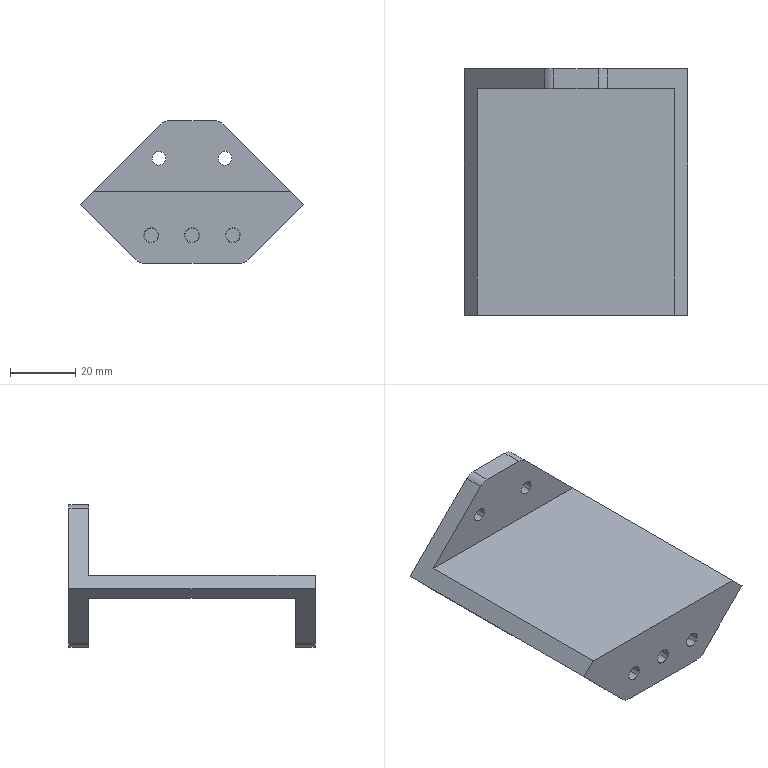NC program | NX | posted with a generic post | part box 68.307 x 75.3 x 43.668 mm
Lines 2926 to 4118 of 6865:
(ZLEVEL_PROFILE_1_COPY_1 , TOOL : D6R0.5)
N5832 T16 M6
N5834 G54
N5836 G17 G0 G90 X-11.309 Y27.842 B0. C0. S9500 M3
N5838 G43 Z30. H16
N5840 Z2.995
N5842 G94 G1 Z-0.005 F3500.
N5844 G3 X-9.487 Y31.148 R3.
N5846 G1 X-9.496 Y31.178
N5848 X-9.541 Y31.65
N5850 Y37.65
N5852 X-9.485 Y38.151
N5854 X-9.538 Y38.15 Z-0.008
N5856 X-9.549 Z-0.01
N5858 X-9.628 Y37.65
N5860 Y31.65
N5862 G3 X-9.55 Y31.15 R3.795
N5864 G1 X-9.633 Z-0.014
N5866 X-9.649 Z-0.019
N5868 X-9.738 Y31.65
N5870 Y37.65
N5872 X-9.648 Y38.15
N5874 X-9.719 Z-0.022
N5876 X-9.718 Z-0.025
N5878 X-9.8 Y37.65
N5880 Y31.65
N5882 G3 X-9.719 Y31.15 R2.274
N5884 G1 X-9.787 Z-0.031
N5886 X-9.852 Y31.65
N5888 Y37.65
N5890 X-9.785 Y38.149
N5892 X-9.833 Y38.15 Z-0.034
N5894 X-9.858 Z-0.038
N5896 X-9.915 Y37.65
N5898 Y31.65
N5900 X-9.857 Y31.15
N5902 X-9.903 Y31.151 Z-0.044
N5904 X-9.919 Z-0.049
N5906 X-9.99 Y31.65
N5908 Y37.65
N5910 X-9.921 Y38.15
N5912 X-9.984 Z-0.056
N5914 X-10.005 Z-0.063
N5916 X-10.077 Y37.65
N5918 Y31.65
N5920 X-10.003 Y31.151
N5922 X-10.104 Z-0.08
N5924 X-10.171 Y31.65
N5926 Y37.65
N5928 X-10.107 Y38.15
N5930 X-10.173 Z-0.089
N5932 X-10.215 Z-0.099
N5934 X-10.269 Y37.65
N5936 Y31.65
N5938 X-10.258 Y31.627
N5940 X-10.227 Y31.203
N5942 X-10.215 Y31.136
N5944 X-10.263 Y31.13 Z-0.11
N5946 X-10.307 Y31.125 Z-0.121
N5948 X-10.363 Y31.65
N5950 Y37.65
N5952 X-10.303 Y38.15
N5954 X-10.308 Y38.256 Z-0.125
N5956 X-10.301 Y38.36 Z-0.129
N5958 X-10.302 Y38.354
N5960 X-10.338 Y38.151
N5962 G3 X-10.399 Y37.65 R2.023
N5964 G1 Y31.65
N5966 X-10.339 Y31.098
N5968 X-10.313 Y31.017
N5970 X-10.356 Y31.015 Z-0.138
N5972 X-10.382 Y31.013 Z-0.147
N5974 X-10.416 Y31.134
N5976 X-10.471 Y31.65
N5978 Y37.65
N5980 X-10.411 Y38.15
N5982 X-10.369 Y38.37
N5984 X-10.314 Y38.541
N5986 X-10.386 Y38.411 Z-0.156
N5988 X-10.456 Y38.282 Z-0.165
N5990 X-10.517 Y38.15 Z-0.174
N5992 X-10.532 Y38.078
N5994 X-10.567 Y37.65
N5996 Y31.65
N5998 X-10.513 Y31.123
N6000 X-10.481 Y31.007
N6002 X-10.551 Y31.074 Z-0.188
N6004 X-10.611 Y31.146 Z-0.202
N6006 X-10.615 Y31.152
N6008 X-10.651 Y31.627
N6010 X-10.663 Y31.65
N6012 Y37.65
N6014 X-10.604 Y38.159
N6016 X-10.659 Y38.167 Z-0.218
N6018 X-10.694 Y38.171 Z-0.233
N6020 X-10.757 Y37.65
N6022 Y31.65
N6024 X-10.746 Y31.627
N6026 X-10.708 Y31.145
N6028 X-10.753 Y31.134 Z-0.249
N6030 X-10.796 Y31.123 Z-0.265
N6032 X-10.851 Y31.65
N6034 Y37.65
N6036 X-10.789 Y38.184
N6038 X-10.832 Y38.189 Z-0.279
N6040 X-10.867 Y38.194 Z-0.292
N6042 X-10.924 Y37.65
N6044 Y31.65
N6046 X-10.867 Y31.105
N6048 X-10.899 Y31.108 Z-0.304
N6050 X-10.92 Y31.109 Z-0.316
N6052 X-10.986 Y31.65
N6054 Y37.65
N6056 X-10.927 Y38.195
N6058 X-10.913 Y38.252
N6060 X-11.012 Y38.218 Z-0.354
N6062 X-11.077 Y37.65
N6064 Y31.65
N6066 X-11.007 Y31.109
N6068 X-11.067 Z-0.373
N6070 X-11.099 Z-0.393
N6072 X-11.168 Y31.65
N6074 Y37.65
N6076 X-11.113 Y38.185
N6078 X-11.209 Y38.153 Z-0.435
N6080 X-11.258 Y37.65
N6082 Y31.65
N6084 X-11.19 Y31.075
N6086 X-11.29 Y31.145 Z-0.478
N6088 X-11.348 Y31.65
N6090 Y37.65
N6092 X-11.292 Y38.156
N6094 X-11.343 Y38.16 Z-0.501
N6096 X-11.377 Y38.163 Z-0.524
N6098 X-11.436 Y37.65
N6100 Y31.65
N6102 X-11.374 Y31.138
N6104 X-11.43 Y31.133 Z-0.548
N6106 X-11.463 Y31.13 Z-0.572
N6108 X-11.524 Y31.65
N6110 Y37.65
N6112 X-11.465 Y38.171
N6114 X-11.516 Y38.175 Z-0.596
N6116 X-11.557 Y38.178 Z-0.621
N6118 X-11.61 Y37.65
N6120 Y31.65
N6122 X-11.567 Y31.174
N6124 X-11.556 Y31.122
N6126 X-11.637 Y31.127 Z-0.673
N6128 X-11.695 Y31.65
N6130 Y37.65
N6132 X-11.638 Y38.173
N6134 X-11.688 Y38.169 Z-0.699
N6136 X-11.721 Y38.166 Z-0.726
N6138 X-11.779 Y37.65
N6140 Y31.65
N6142 X-11.72 Y31.134
N6144 X-11.773 Y31.139 Z-0.754
N6146 X-11.806 Y31.142 Z-0.781
N6148 X-11.862 Y31.65
N6150 Y37.65
N6152 X-11.806 Y38.159
N6154 X-11.858 Y38.154 Z-0.81
N6156 X-11.895 Y38.151 Z-0.838
N6158 X-11.944 Y37.65
N6160 Y31.65
N6162 X-11.913 Y31.238
N6164 X-11.895 Y31.149
N6166 X-11.94 Y31.15 Z-0.868
N6168 X-11.973 Z-0.897
N6170 X-12.025 Y31.65
N6172 Y37.65
N6174 X-11.972 Y38.15
N6176 X-12.019 Z-0.927
N6178 X-12.048 Z-0.958
N6180 X-12.104 Y37.65
N6182 Y31.65
N6184 X-12.053 Y31.15
N6186 X-12.097 Z-0.989
N6188 X-12.133 Y31.149 Z-1.02
N6190 X-12.181 Y31.65
N6192 Y37.65
N6194 X-12.126 Y38.15
N6196 X-12.175 Z-1.052
N6198 X-12.207 Z-1.084
N6200 X-12.258 Y37.65
N6202 Y31.65
N6204 X-12.212 Y31.15
N6206 X-12.25 Z-1.117
N6208 X-12.288 Z-1.15
N6210 X-12.333 Y31.65
N6212 Y37.65
N6214 X-12.285 Y38.15
N6216 X-12.324 Z-1.183
N6218 X-12.359 Z-1.216
N6220 X-12.405 Y37.65
N6222 Y31.65
N6224 X-12.364 Y31.149
N6226 X-12.395 Y31.15 Z-1.249
N6228 X-12.43 Z-1.281
N6230 X-12.473 Y31.65
N6232 Y37.65
N6234 X-12.431 Y38.15
N6236 X-12.477 Z-1.315
N6238 X-12.507 Z-1.349
N6240 X-12.542 Y37.65
N6242 Y31.65
N6244 X-12.506 Y31.149
N6246 X-12.539 Y31.15 Z-1.384
N6248 X-12.579 Z-1.419
N6250 X-12.612 Y31.65
N6252 Y37.65
N6254 X-12.584 Y38.15
N6256 X-12.62 Z-1.454
N6258 X-12.658 Z-1.49
N6260 X-12.682 Y37.65
N6262 Y31.65
N6264 X-12.652 Y31.15
N6266 X-12.685 Z-1.525
N6268 X-12.724 Z-1.561
N6270 X-12.753 Y31.65
N6272 Y37.65
N6274 X-12.73 Y38.15
N6276 X-12.764 Z-1.596
N6278 X-12.802 Z-1.631
N6280 X-12.824 Y37.65
N6282 Y31.627
N6284 X-12.796 Y31.15
N6286 X-12.83 Z-1.667
N6288 X-12.868 Z-1.702
N6290 X-12.894 Y31.627
N6292 Y37.65
N6294 X-12.874 Y38.15
N6296 X-12.908 Z-1.737
N6298 X-12.945 Z-1.773
N6300 X-12.965 Y37.65
N6302 Y31.65
N6304 X-12.941 Y31.15
N6306 X-12.976 Z-1.808
N6308 X-13.013 Z-1.843
N6310 X-13.036 Y31.65
N6312 Y37.65
N6314 X-13.018 Y38.15
N6316 X-13.053 Z-1.879
N6318 X-13.09 Z-1.914
N6320 X-13.106 Y37.65
N6322 Y31.65
N6324 X-13.085 Y31.15
N6326 X-13.121 Z-1.949
N6328 X-13.157 Z-1.985
N6330 X-13.177 Y31.65
N6332 Y37.65
N6334 X-13.162 Y38.15
N6336 X-13.197 Z-2.02
N6338 X-13.234 Z-2.056
N6340 X-13.248 Y37.65
N6342 Y31.65
N6344 X-13.229 Y31.15
N6346 X-13.266 Z-2.091
N6348 X-13.302 Z-2.126
N6350 X-13.319 Y31.65
N6352 Y37.65
N6354 X-13.306 Y38.15
N6356 X-13.341 Z-2.162
N6358 X-13.378 Z-2.197
N6360 X-13.389 Y37.65
N6362 Y31.627
N6364 X-13.373 Y31.15
N6366 X-13.411 Z-2.232
N6368 X-13.445 Z-2.268
N6370 X-13.46 Y31.65
N6372 Y37.65
N6374 X-13.45 Y38.15
N6376 X-13.486 Z-2.303
N6378 X-13.522 Z-2.338
N6380 X-13.531 Y37.65
N6382 Y31.65
N6384 X-13.517 Y31.15
N6386 X-13.555 Z-2.374
N6388 X-13.589 Z-2.409
N6390 X-13.601 Y31.65
N6392 Y37.65
N6394 X-13.594 Y38.15
N6396 X-13.63 Z-2.444
N6398 X-13.665 Z-2.48
N6400 X-13.672 Y37.65
N6402 Y31.65
N6404 X-13.661 Y31.15
N6406 X-13.7 Z-2.515
N6408 X-13.733 Z-2.55
N6410 X-13.743 Y31.65
N6412 Y37.65
N6414 X-13.737 Y38.15
N6416 X-13.774 Z-2.586
N6418 X-13.809 Z-2.621
N6420 X-13.814 Y37.65
N6422 Y31.65
N6424 X-13.805 Y31.15
N6426 X-13.844 Z-2.657
N6428 X-13.876 Z-2.692
N6430 X-13.884 Y31.65
N6432 Y37.65
N6434 X-13.881 Y38.15
N6436 X-13.917 Z-2.727
N6438 X-13.952 Z-2.763
N6440 X-13.955 Y37.65
N6442 Y31.65
N6444 X-13.948 Y31.15
N6446 X-13.986 Z-2.798
N6448 X-14.019 Z-2.833
N6450 X-14.026 Y31.65
N6452 Y37.65
N6454 X-14.023 Y38.15
N6456 X-14.059 Z-2.869
N6458 X-14.094 Z-2.904
N6460 X-14.096 Y37.65
N6462 Y31.65
N6464 X-14.09 Y31.15
N6466 X-14.128 Z-2.939
N6468 X-14.161 Z-2.975
N6470 X-14.167 Y31.65
N6472 Y37.65
N6474 X-14.165 Y38.15
N6476 X-14.201 Z-3.01
N6478 X-14.236 Z-3.045
N6480 X-14.238 Y37.65
N6482 Y31.65
N6484 X-14.232 Y31.15
N6486 X-14.27 Z-3.081
N6488 X-14.303 Z-3.116
N6490 X-14.309 Y31.65
N6492 Y37.65
N6494 X-14.307 Y38.15
N6496 X-14.342 Z-3.152
N6498 X-14.377 Z-3.187
N6500 X-14.379 Y37.65
N6502 Y31.65
N6504 X-14.374 Y31.15
N6506 X-14.412 Z-3.222
N6508 X-14.445 Z-3.258
N6510 X-14.45 Y31.65
N6512 Y37.65
N6514 X-14.448 Y38.15
N6516 X-14.484 Z-3.293
N6518 X-14.519 Z-3.328
N6520 X-14.521 Y37.65
N6522 Y31.65
N6524 X-14.516 Y31.15
N6526 X-14.554 Z-3.364
N6528 X-14.587 Z-3.399
N6530 X-14.591 Y31.65
N6532 Y37.65
N6534 X-14.59 Y38.15
N6536 X-14.626 Z-3.434
N6538 X-14.661 Z-3.47
N6540 X-14.662 Y37.65
N6542 Y31.65
N6544 X-14.658 Y31.15
N6546 X-14.696 Z-3.505
N6548 X-14.728 Z-3.54
N6550 X-14.733 Y31.65
N6552 Y37.65
N6554 X-14.732 Y38.15
N6556 X-14.767 Z-3.576
N6558 X-14.802 Z-3.611
N6560 X-14.804 Y37.65
N6562 Y31.65
N6564 X-14.799 Y31.15
N6566 X-14.837 Z-3.647
N6568 X-14.87 Z-3.682
N6570 X-14.874 Y31.65
N6572 Y37.65
N6574 X-14.873 Y38.15
N6576 X-14.909 Z-3.717
N6578 X-14.944 Z-3.753
N6580 X-14.945 Y37.65
N6582 Y31.65
N6584 X-14.941 Y31.15
N6586 X-14.979 Z-3.788
N6588 X-15.012 Z-3.823
N6590 X-15.016 Y31.65
N6592 Y37.65
N6594 X-15.015 Y38.15
N6596 X-15.051 Z-3.859
N6598 X-15.086 Z-3.894
N6600 Y37.65
N6602 Y31.65
N6604 X-15.083 Y31.15
N6606 X-15.121 Z-3.929
N6608 X-15.153 Z-3.965
N6610 X-15.157 Y31.65
N6612 Y37.65
N6614 X-15.156 Y38.15
N6616 X-15.192 Z-4.
N6618 X-15.227 Z-4.035
N6620 X-15.228 Y37.65
N6622 Y31.65
N6624 X-15.224 Y31.15
N6626 X-15.263 Z-4.071
N6628 X-15.295 Z-4.106
N6630 X-15.299 Y31.65
N6632 Y37.65
N6634 X-15.298 Y38.15
N6636 X-15.334 Z-4.141
N6638 X-15.369 Z-4.177
N6640 Y37.65
N6642 Y31.65
N6644 X-15.367 Y31.15
N6646 X-15.404 Z-4.212
N6648 X-15.437 Z-4.248
N6650 X-15.44 Y31.65
N6652 Y37.65
N6654 Y38.15
N6656 X-15.475 Z-4.283
N6658 X-15.51 Z-4.318
N6660 X-15.511 Y37.65
N6662 Y31.65
N6664 X-15.507 Y31.15
N6666 X-15.546 Z-4.354
N6668 X-15.578 Z-4.389
N6670 X-15.581 Y31.65
N6672 Y37.65
N6674 Y38.15
N6676 X-15.617 Z-4.424
N6678 X-15.652 Z-4.46
N6680 Y37.65
N6682 Y31.65
N6684 X-15.649 Y31.15
N6686 X-15.687 Z-4.495
N6688 X-15.72 Z-4.53
N6690 X-15.723 Y31.65
N6692 Y37.65
N6694 X-15.722 Y38.15
N6696 X-15.758 Z-4.566
N6698 X-15.793 Z-4.601
N6700 Y37.65
N6702 Y31.65
N6704 X-15.79 Y31.15
N6706 X-15.829 Z-4.636
N6708 X-15.861 Z-4.672
N6710 X-15.864 Y31.65
N6712 Y37.65
N6714 Y38.15
N6716 X-15.899 Z-4.707
N6718 X-15.935 Z-4.743
N6720 Y37.65
N6722 Y31.65
N6724 X-15.932 Y31.15
N6726 X-15.97 Z-4.778
N6728 X-16.002 Z-4.813
N6730 X-16.006 Y31.65
N6732 Y37.65
N6734 X-16.005 Y38.15
N6736 X-16.041 Z-4.849
N6738 X-16.076 Z-4.884
N6740 Y37.65
N6742 Y31.65
N6744 X-16.073 Y31.15
N6746 X-16.112 Z-4.919
N6748 X-16.144 Z-4.955
N6750 X-16.147 Y31.65
N6752 Y37.65
N6754 Y38.15
N6756 X-16.182 Z-4.99
N6758 X-16.217 Z-5.025
N6760 X-16.218 Y37.65
N6762 Y31.65
N6764 X-16.215 Y31.15
N6766 X-16.253 Z-5.061
N6768 X-16.285 Z-5.096
N6770 X-16.288 Y31.65
N6772 Y37.65
N6774 Y38.15
N6776 X-16.324 Z-5.131
N6778 X-16.359 Z-5.167
N6780 Y37.65
N6782 Y31.65
N6784 X-16.356 Y31.15
N6786 X-16.394 Z-5.202
N6788 X-16.427 Z-5.237
N6790 X-16.43 Y31.65
N6792 Y37.65
N6794 Y38.15
N6796 X-16.465 Z-5.273
N6798 X-16.5 Z-5.308
N6800 X-16.501 Y37.65
N6802 Y31.65
N6804 X-16.498 Y31.15
N6806 X-16.536 Z-5.344
N6808 X-16.568 Z-5.379
N6810 X-16.571 Y31.65
N6812 Y37.65
N6814 Y38.15
N6816 X-16.607 Z-5.414
N6818 X-16.642 Z-5.45
N6820 Y37.65
N6822 Y31.65
N6824 X-16.639 Y31.15
N6826 X-16.677 Z-5.485
N6828 X-16.71 Z-5.52
N6830 X-16.713 Y31.65
N6832 Y37.65
N6834 X-16.712 Y38.15
N6836 X-16.748 Z-5.556
N6838 X-16.783 Z-5.591
N6840 Y37.65
N6842 Y31.65
N6844 X-16.78 Y31.15
N6846 X-16.819 Z-5.626
N6848 X-16.851 Z-5.662
N6850 X-16.854 Y31.65
N6852 Y37.65
N6854 Y38.15
N6856 X-16.889 Z-5.697
N6858 X-16.925 Z-5.732
N6860 Y37.65
N6862 Y31.65
N6864 X-16.922 Y31.15
N6866 X-16.96 Z-5.768
N6868 X-16.993 Z-5.803
N6870 X-16.996 Y31.65
N6872 Y37.65
N6874 X-16.995 Y38.15
N6876 X-17.031 Z-5.839
N6878 X-17.066 Z-5.874
N6880 Y37.65
N6882 Y31.65
N6884 X-17.063 Y31.15
N6886 X-17.102 Z-5.909
N6888 X-17.134 Z-5.945
N6890 X-17.137 Y31.65
N6892 Y37.65
N6894 Y38.15
N6896 X-17.172 Z-5.98
N6898 X-17.207 Z-6.015
N6900 X-17.208 Y37.65
N6902 Y31.65
N6904 X-17.205 Y31.15
N6906 X-17.243 Z-6.051
N6908 X-17.275 Z-6.086
N6910 X-17.278 Y31.65
N6912 Y37.65
N6914 Y38.15
N6916 X-17.314 Z-6.121
N6918 X-17.349 Z-6.157
N6920 Y37.65
N6922 Y31.65
N6924 X-17.346 Y31.15
N6926 X-17.384 Z-6.192
N6928 X-17.417 Z-6.227
N6930 X-17.42 Y31.65
N6932 Y37.65
N6934 Y38.15
N6936 X-17.455 Z-6.263
N6938 X-17.49 Z-6.298
N6940 X-17.491 Y37.65
N6942 Y31.65
N6944 X-17.487 Y31.15
N6946 X-17.526 Z-6.334
N6948 X-17.558 Z-6.369
N6950 X-17.561 Y31.65
N6952 Y37.65
N6954 Y38.15
N6956 X-17.597 Z-6.404
N6958 X-17.632 Z-6.44
N6960 Y37.65
N6962 Y31.65
N6964 X-17.629 Y31.15
N6966 X-17.667 Z-6.475
N6968 X-17.7 Z-6.51
N6970 X-17.703 Y31.65
N6972 Y37.65
N6974 X-17.702 Y38.15
N6976 X-17.738 Z-6.546
N6978 X-17.773 Z-6.581
N6980 Y37.65
N6982 Y31.65
N6984 X-17.77 Y31.15
N6986 X-17.809 Z-6.616
N6988 X-17.841 Z-6.652
N6990 X-17.844 Y31.65
N6992 Y37.65
N6994 Y38.15
N6996 X-17.879 Z-6.687
N6998 X-17.914 Z-6.722
N7000 X-17.915 Y37.65
N7002 Y31.65
N7004 X-17.912 Y31.15
N7006 X-17.95 Z-6.758
N7008 X-17.982 Z-6.793
N7010 X-17.986 Y31.65
N7012 Y37.65
N7014 X-17.985 Y38.15
N7016 X-18.021 Z-6.828
N7018 X-18.056 Z-6.864
N7020 Y37.65
N7022 Y31.65
N7024 X-18.053 Y31.15
N7026 X-18.092 Z-6.899
N7028 X-18.124 Z-6.935
N7030 X-18.127 Y31.65
N7032 Y37.65
N7034 Y38.15
N7036 X-18.162 Z-6.97
N7038 X-18.197 Z-7.005
N7040 X-18.198 Y37.65
N7042 Y31.65
N7044 X-18.195 Y31.15
N7046 X-18.233 Z-7.041
N7048 X-18.265 Z-7.076
N7050 X-18.268 Y31.65
N7052 Y37.65
N7054 Y38.15
N7056 X-18.304 Z-7.111
N7058 X-18.339 Z-7.147
N7060 Y37.65
N7062 Y31.65
N7064 X-18.336 Y31.15
N7066 X-18.374 Z-7.182
N7068 X-18.407 Z-7.217
N7070 X-18.41 Y31.65
N7072 Y37.65
N7074 X-18.409 Y38.15
N7076 X-18.445 Z-7.253
N7078 X-18.48 Z-7.288
N7080 Y37.65
N7082 Y31.65
N7084 X-18.478 Y31.15
N7086 X-18.516 Z-7.323
N7088 X-18.548 Z-7.359
N7090 X-18.551 Y31.65
N7092 Y37.65
N7094 Y38.15
N7096 X-18.587 Z-7.394
N7098 X-18.622 Z-7.43
N7100 Y37.65
N7102 Y31.65
N7104 X-18.619 Y31.15
N7106 X-18.657 Z-7.465
N7108 X-18.69 Z-7.5
N7110 X-18.693 Y31.65
N7112 Y37.65
N7114 X-18.692 Y38.15
N7116 X-18.728 Z-7.536
N7118 X-18.763 Z-7.571
N7120 Y37.65
N7122 Y31.65
N7124 X-18.76 Y31.15
N7126 X-18.799 Z-7.606
N7128 X-18.831 Z-7.642
N7130 X-18.834 Y31.65
N7132 Y37.65
N7134 Y38.15
N7136 X-18.869 Z-7.677
N7138 X-18.904 Z-7.712
N7140 X-18.905 Y37.65
N7142 Y31.65
N7144 X-18.902 Y31.15
N7146 X-18.94 Z-7.748
N7148 X-18.972 Z-7.783
N7150 X-18.975 Y31.65
N7152 Y37.65
N7154 Y38.15
N7156 X-19.011 Z-7.818
N7158 X-19.046 Z-7.854
N7160 Y37.65
N7162 Y31.65
N7164 X-19.043 Y31.15
N7166 X-19.082 Z-7.889
N7168 X-19.114 Z-7.924
N7170 X-19.117 Y31.65
N7172 Y37.65
N7174 Y38.15
N7176 X-19.152 Z-7.96
N7178 X-19.187 Z-7.995
N7180 X-19.188 Y37.65
N7182 Y31.65
N7184 X-19.185 Y31.15
N7186 X-19.223 Z-8.031
N7188 X-19.255 Z-8.066
N7190 X-19.258 Y31.65
N7192 Y37.65
N7194 Y38.15
N7196 X-19.294 Z-8.101
N7198 X-19.329 Z-8.137
N7200 Y37.65
N7202 Y31.65
N7204 X-19.326 Y31.15
N7206 X-19.364 Z-8.172
N7208 X-19.397 Z-8.207
N7210 X-19.4 Y31.65
N7212 Y37.65
N7214 X-19.399 Y38.15
N7216 X-19.435 Z-8.243
N7218 X-19.47 Z-8.278
N7220 Y37.65
N7222 Y31.65
N7224 X-19.467 Y31.15
N7226 X-19.506 Z-8.313
N7228 X-19.538 Z-8.349
N7230 X-19.541 Y31.65
N7232 Y37.65
N7234 Y38.15
N7236 X-19.577 Z-8.384
N7238 X-19.612 Z-8.419
N7240 Y37.65
N7242 Y31.65
N7244 X-19.609 Y31.15
N7246 X-19.647 Z-8.455
N7248 X-19.68 Z-8.49
N7250 X-19.683 Y31.65
N7252 Y37.65
N7254 X-19.682 Y38.15
N7256 X-19.718 Z-8.526
N7258 X-19.753 Z-8.561
N7260 Y37.65
N7262 Y31.65
N7264 X-19.75 Y31.15
N7266 X-19.789 Z-8.596
N7268 X-19.821 Z-8.632
N7270 X-19.824 Y31.65
N7272 Y37.65
N7274 Y38.15
N7276 X-19.859 Z-8.667
N7278 X-19.894 Z-8.702
N7280 X-19.895 Y37.65
N7282 Y31.65
N7284 X-19.892 Y31.15
N7286 X-19.93 Z-8.738
N7288 X-19.962 Z-8.773
N7290 X-19.965 Y31.65
N7292 Y37.65
N7294 Y38.15
N7296 X-20.001 Z-8.808
N7298 X-20.036 Z-8.844
N7300 Y37.65
N7302 Y31.65
N7304 X-20.033 Y31.15
N7306 X-20.071 Z-8.879
N7308 X-20.104 Z-8.914
N7310 X-20.107 Y31.65
N7312 Y37.65
N7314 Y38.15
N7316 X-20.142 Z-8.95
N7318 X-20.177 Z-8.985
N7320 X-20.178 Y37.65
N7322 Y31.65
N7324 X-20.174 Y31.15
N7326 X-20.213 Z-9.021
N7328 X-20.245 Z-9.056
N7330 X-20.248 Y31.65
N7332 Y37.65
N7334 Y38.15
N7336 X-20.284 Z-9.091
N7338 X-20.319 Z-9.127
N7340 Y37.65
N7342 Y31.65
N7344 X-20.316 Y31.15
N7346 X-20.354 Z-9.162
N7348 X-20.387 Z-9.197
N7350 X-20.39 Y31.65
N7352 Y37.65
N7354 X-20.389 Y38.15
N7356 X-20.425 Z-9.233
N7358 X-20.46 Z-9.268
N7360 Y37.65
N7362 Y31.65
N7364 X-20.457 Y31.15
N7366 X-20.496 Z-9.303
N7368 X-20.528 Z-9.339
N7370 X-20.531 Y31.65
N7372 Y37.65
N7374 Y38.15
N7376 X-20.566 Z-9.374
N7378 X-20.602 Z-9.409
N7380 Y37.65
N7382 Y31.65
N7384 X-20.599 Y31.15
N7386 X-20.637 Z-9.445
N7388 X-20.669 Z-9.48
N7390 X-20.673 Y31.65
N7392 Y37.65
N7394 X-20.672 Y38.15
N7396 X-20.708 Z-9.515
N7398 X-20.743 Z-9.551
N7400 Y37.65
N7402 Y31.65
N7404 X-20.74 Y31.15
N7406 X-20.779 Z-9.586
N7408 X-20.811 Z-9.622
N7410 X-20.814 Y31.65
N7412 Y37.65
N7414 Y38.15
N7416 X-20.849 Z-9.657
N7418 X-20.884 Z-9.692
N7420 X-20.885 Y37.65
N7422 Y31.65
N7424 X-20.882 Y31.15
N7426 X-20.92 Z-9.728
N7428 X-20.952 Z-9.763
N7430 X-20.955 Y31.65
N7432 Y37.65
N7434 Y38.15
N7436 X-20.991 Z-9.798
N7438 X-21.026 Z-9.834
N7440 Y37.65
N7442 Y31.65
N7444 X-21.023 Y31.15
N7446 X-21.061 Z-9.869
N7448 X-21.094 Z-9.904
N7450 X-21.097 Y31.65
N7452 Y37.65
N7454 X-21.096 Y38.15
N7456 X-21.132 Z-9.94
N7458 X-21.167 Z-9.975
N7460 Y37.65
N7462 Y31.65
N7464 X-21.164 Y31.15
N7466 X-21.203 Z-10.01
N7468 X-21.237 Z-10.046
N7470 X-21.238 Y31.65
N7472 Y37.65
N7474 Y38.15
N7476 X-21.274 Z-10.081
N7478 X-21.309 Z-10.117
N7480 Y37.65
N7482 Y31.65
N7484 X-21.306 Y31.15
N7486 X-21.344 Z-10.152
N7488 X-21.377 Z-10.187
N7490 X-21.38 Y31.65
N7492 Y37.65
N7494 X-21.379 Y38.15
N7496 X-21.415 Z-10.223
N7498 X-21.45 Z-10.258
N7500 Y37.65
N7502 Y31.65
N7504 X-21.447 Y31.15
N7506 X-21.486 Z-10.293
N7508 X-21.518 Z-10.329
N7510 X-21.521 Y31.65
N7512 Y37.65
N7514 Y38.15
N7516 X-21.556 Z-10.364
N7518 X-21.591 Z-10.399
N7520 X-21.592 Y37.65
N7522 Y31.65
N7524 X-21.589 Y31.15
N7526 X-21.627 Z-10.435
N7528 X-21.659 Z-10.47
N7530 X-21.662 Y31.65
N7532 Y37.65
N7534 Y38.15
N7536 X-21.698 Z-10.505
N7538 X-21.733 Z-10.541
N7540 Y37.65
N7542 Y31.65
N7544 X-21.73 Y31.15
N7546 X-21.769 Z-10.576
N7548 X-21.801 Z-10.612
N7550 X-21.804 Y31.65
N7552 Y37.65
N7554 Y38.15
N7556 X-21.839 Z-10.647
N7558 X-21.874 Z-10.682
N7560 X-21.875 Y37.65
N7562 Y31.65
N7564 X-21.872 Y31.15
N7566 X-21.91 Z-10.718
N7568 X-21.942 Z-10.753
N7570 X-21.945 Y31.65
N7572 Y37.65
N7574 Y38.15
N7576 X-21.981 Z-10.788
N7578 X-22.016 Z-10.824
N7580 Y37.65
N7582 Y31.65
N7584 X-22.013 Y31.15
N7586 X-22.051 Z-10.859
N7588 X-22.084 Z-10.894
N7590 X-22.087 Y31.65
N7592 Y37.65
N7594 X-22.086 Y38.15
N7596 X-22.122 Z-10.93
N7598 X-22.157 Z-10.965
N7600 Y37.65
N7602 Y31.65
N7604 X-22.154 Y31.15
N7606 X-22.193 Z-11.
N7608 X-22.225 Z-11.036
N7610 X-22.228 Y31.65
N7612 Y37.65
N7614 Y38.15
N7616 X-22.264 Z-11.071
N7618 X-22.299 Z-11.106
N7620 Y37.65
N7622 Y31.65
N7624 X-22.296 Y31.15
N7626 X-22.334 Z-11.142
N7628 X-22.367 Z-11.177
N7630 X-22.37 Y31.65
N7632 Y37.65
N7634 X-22.369 Y38.15
N7636 X-22.405 Z-11.213
N7638 X-22.44 Z-11.248
N7640 Y37.65
N7642 Y31.65
N7644 X-22.437 Y31.15
N7646 X-22.476 Z-11.283
N7648 X-22.508 Z-11.319
N7650 X-22.511 Y31.65
N7652 Y37.65
N7654 Y38.15
N7656 X-22.546 Z-11.354
N7658 X-22.581 Z-11.389
N7660 X-22.582 Y37.65
N7662 Y31.65
N7664 X-22.579 Y31.15
N7666 X-22.617 Z-11.425
N7668 X-22.649 Z-11.46
N7670 X-22.652 Y31.65
N7672 Y37.65
N7674 Y38.15
N7676 X-22.688 Z-11.495
N7678 X-22.723 Z-11.531
N7680 Y37.65
N7682 Y31.65
N7684 X-22.72 Y31.15
N7686 X-22.758 Z-11.566
N7688 X-22.791 Z-11.601
N7690 X-22.794 Y31.65
N7692 Y37.65
N7694 Y38.15
N7696 X-22.829 Z-11.637
N7698 X-22.864 Z-11.672
N7700 X-22.865 Y37.65
N7702 Y31.65
N7704 X-22.861 Y31.15
N7706 X-22.9 Z-11.708
N7708 X-22.932 Z-11.743
N7710 X-22.935 Y31.65
N7712 Y37.65
N7714 Y38.15
N7716 X-22.971 Z-11.778
N7718 X-23.006 Z-11.814
N7720 Y37.65
N7722 Y31.65
N7724 X-23.003 Y31.15
N7726 X-23.041 Z-11.849
N7728 X-23.074 Z-11.884
N7730 X-23.077 Y31.65
N7732 Y37.65
N7734 X-23.076 Y38.15
N7736 X-23.112 Z-11.92
N7738 X-23.147 Z-11.955
N7740 Y37.65
N7742 Y31.65
N7744 X-23.144 Y31.15
N7746 X-23.183 Z-11.99
N7748 X-23.215 Z-12.026
N7750 X-23.218 Y31.65
N7752 Y37.65
N7754 Y38.15
N7756 X-23.253 Z-12.061
N7758 X-23.289 Z-12.096
N7760 Y37.65
N7762 Y31.65
N7764 X-23.286 Y31.15
N7766 X-23.324 Z-12.132
N7768 X-23.356 Z-12.167
N7770 X-23.36 Y31.65
N7772 Y37.65
N7774 X-23.359 Y38.15
N7776 X-23.395 Z-12.202
N7778 X-23.43 Z-12.238
N7780 Y37.65
N7782 Y31.65
N7784 X-23.427 Y31.15
N7786 X-23.466 Z-12.273
N7788 X-23.498 Z-12.309
N7790 X-23.501 Y31.65
N7792 Y37.65
N7794 Y38.15
N7796 X-23.536 Z-12.344
N7798 X-23.571 Z-12.379
N7800 X-23.572 Y37.65
N7802 Y31.65
N7804 X-23.569 Y31.15
N7806 X-23.607 Z-12.415
N7808 X-23.639 Z-12.45
N7810 X-23.642 Y31.65
N7812 Y37.65
N7814 Y38.15
N7816 X-23.678 Z-12.485
N7818 X-23.713 Z-12.521
N7820 Y37.65
N7822 Y31.65
N7824 X-23.71 Y31.15
N7826 X-23.748 Z-12.556
N7828 X-23.781 Z-12.591
N7830 X-23.784 Y31.65
N7832 Y37.65
N7834 X-23.783 Y38.15
N7836 X-23.819 Z-12.627
N7838 X-23.854 Z-12.662
N7840 X-23.855 Y37.65
N7842 Y31.65
N7844 X-23.851 Y31.15
N7846 X-23.89 Z-12.697
N7848 X-23.922 Z-12.733
N7850 X-23.925 Y31.65
N7852 Y37.65
N7854 Y38.15
N7856 X-23.961 Z-12.768
N7858 X-23.996 Z-12.804
N7860 Y37.65
N7862 Y31.65
N7864 X-23.993 Y31.15
N7866 X-24.031 Z-12.839
N7868 X-24.064 Z-12.874
N7870 X-24.067 Y31.65
N7872 Y37.65
N7874 X-24.066 Y38.15
N7876 X-24.102 Z-12.91
N7878 X-24.137 Z-12.945
N7880 Y37.65
N7882 Y31.65
N7884 X-24.134 Y31.15
N7886 X-24.173 Z-12.98
N7888 X-24.205 Z-13.016
N7890 X-24.208 Y31.65
N7892 Y37.65
N7894 Y38.15
N7896 X-24.243 Z-13.051
N7898 X-24.278 Z-13.086
N7900 X-24.279 Y37.65
N7902 Y31.65
N7904 X-24.276 Y31.15
N7906 X-24.314 Z-13.122
N7908 X-24.347 Z-13.157
N7910 X-24.349 Y31.65
N7912 Y37.65
N7914 Y38.15
N7916 X-24.385 Z-13.192
N7918 X-24.42 Z-13.228
N7920 Y37.65
N7922 Y31.65
N7924 X-24.417 Y31.15
N7926 X-24.456 Z-13.263
N7928 X-24.488 Z-13.299
N7930 X-24.491 Y31.65
N7932 Y37.65
N7934 Y38.15
N7936 X-24.526 Z-13.334
N7938 X-24.561 Z-13.369
N7940 X-24.562 Y37.65
N7942 Y31.65
N7944 X-24.559 Y31.15
N7946 X-24.597 Z-13.405
N7948 X-24.629 Z-13.44
N7950 X-24.632 Y31.65
N7952 Y37.65
N7954 Y38.15
N7956 X-24.668 Z-13.475
N7958 X-24.703 Z-13.511
N7960 Y37.65
N7962 Y31.65
N7964 X-24.7 Y31.15
N7966 X-24.738 Z-13.546
N7968 X-24.771 Z-13.581
N7970 X-24.774 Y31.65
N7972 Y37.65
N7974 X-24.773 Y38.15
N7976 X-24.809 Z-13.617
N7978 X-24.844 Z-13.652
N7980 Y37.65
N7982 Y31.65
N7984 X-24.841 Y31.15
N7986 X-24.88 Z-13.687
N7988 X-24.912 Z-13.723
N7990 X-24.915 Y31.65
N7992 Y37.65
N7994 Y38.15
N7996 X-24.951 Z-13.758
N7998 X-24.986 Z-13.793
N8000 Y37.65
N8002 Y31.65
N8004 X-24.983 Y31.15
N8006 X-25.021 Z-13.829
N8008 X-25.054 Z-13.864
N8010 X-25.057 Y31.65
N8012 Y37.65
N8014 X-25.056 Y38.15
N8016 X-25.092 Z-13.9
N8018 X-25.127 Z-13.935
N8020 Y37.65
N8022 Y31.65
N8024 X-25.124 Y31.15
N8026 X-25.163 Z-13.97
N8028 X-25.195 Z-14.006
N8030 X-25.198 Y31.65
N8032 Y37.65
N8034 Y38.15
N8036 X-25.233 Z-14.041
N8038 X-25.268 Z-14.076
N8040 X-25.269 Y37.65
N8042 Y31.65
N8044 X-25.266 Y31.15
N8046 X-25.304 Z-14.112
N8048 X-25.336 Z-14.147
N8050 X-25.339 Y31.65
N8052 Y37.65
N8054 Y38.15
N8056 X-25.375 Z-14.182
N8058 X-25.41 Z-14.218
N8060 Y37.65
N8062 Y31.65
N8064 X-25.407 Y31.15
N8066 X-25.445 Z-14.253
N8068 X-25.478 Z-14.288
N8070 X-25.481 Y31.65
N8072 Y37.65
N8074 Y38.15
N8076 X-25.516 Z-14.324
N8078 X-25.551 Z-14.359
N8080 X-25.552 Y37.65
N8082 Y31.65
N8084 X-25.549 Y31.15
N8086 X-25.587 Z-14.395
N8088 X-25.619 Z-14.43
N8090 X-25.622 Y31.65
N8092 Y37.65
N8094 Y38.15
N8096 X-25.658 Z-14.465
N8098 X-25.693 Z-14.501
N8100 Y37.65
N8102 Y31.65
N8104 X-25.69 Y31.15
N8106 X-25.728 Z-14.536
N8108 X-25.761 Z-14.571
N8110 X-25.764 Y31.65
N8112 Y37.65
N8114 X-25.763 Y38.15
N8116 X-25.799 Z-14.607
N8118 X-25.834 Z-14.642
N8120 Y37.65
N8122 Y31.65
N8124 X-25.831 Y31.15
N8126 X-25.87 Z-14.677
N8128 X-25.902 Z-14.713
N8130 X-25.905 Y31.65
N8132 Y37.65
N8134 Y38.15
N8136 X-25.94 Z-14.748
N8138 X-25.976 Z-14.783
N8140 Y37.65
N8142 Y31.65
N8144 X-25.973 Y31.15
N8146 X-26.011 Z-14.819
N8148 X-26.043 Z-14.854
N8150 X-26.047 Y31.65
N8152 Y37.65
N8154 X-26.046 Y38.15
N8156 X-26.082 Z-14.89
N8158 X-26.117 Z-14.925
N8160 Y37.65
N8162 Y31.65
N8164 X-26.114 Y31.15
N8166 X-26.153 Z-14.96
N8168 X-26.185 Z-14.996
N8170 X-26.188 Y31.65
N8172 Y37.65
N8174 Y38.15
N8176 X-26.223 Z-15.031
N8178 X-26.258 Z-15.066
N8180 X-26.259 Y37.65
N8182 Y31.65
N8184 X-26.256 Y31.15
N8186 X-26.294 Z-15.102
N8188 X-26.326 Z-15.137
N8190 X-26.329 Y31.65
N8192 Y37.65
N8194 Y38.15
N8196 X-26.365 Z-15.172
N8198 X-26.4 Z-15.208
N8200 Y37.65
N8202 Y31.65
N8204 X-26.397 Y31.15
N8206 X-26.435 Z-15.243
N8208 X-26.468 Z-15.278
N8210 X-26.471 Y31.65